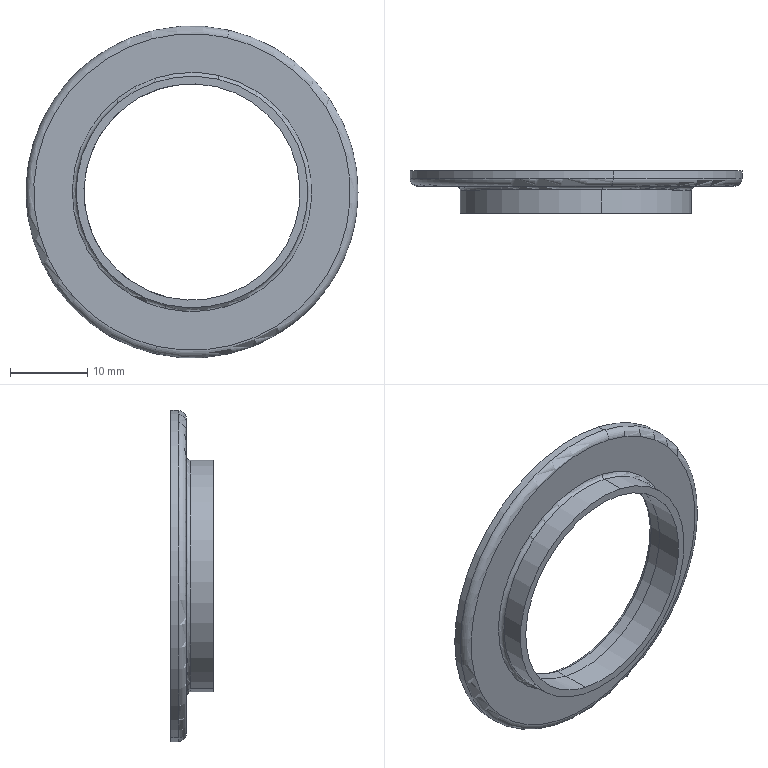Part | SolidWorks | features BaseBody 1 | 1 solid | 17 faces | box 43 x 5.5 x 43 mm | volume 1963 mm3 | cylinder 8 | torus 6 | plane 3 | commonest cylinder face diameters 28 x4 30 x2 43 x2
STEP:
#1=CARTESIAN_POINT('',(1957.589,243.9,872.98));
#2=VERTEX_POINT('',#1);
#3=CARTESIAN_POINT('',(1948.411,243.9,833.02));
#4=VERTEX_POINT('',#3);
#5=CARTESIAN_POINT('',(1953.,243.9,853.));
#6=DIRECTION('',(0.,1.,0.));
#7=DIRECTION('',(-0.9746,0.,0.2239));
#8=AXIS2_PLACEMENT_3D('',#5,#6,#7);
#9=CIRCLE('',#8,20.5);
#10=EDGE_CURVE('',#2,#4,#9,.T.);
#11=ORIENTED_EDGE('',*,*,#10,.F.);
#12=CARTESIAN_POINT('',(1957.589,243.9,872.98));
#13=CARTESIAN_POINT('',(1955.644,243.9,873.427));
#14=CARTESIAN_POINT('',(1953.644,243.9,873.637));
#15=CARTESIAN_POINT('',(1951.628,243.9,873.601));
#16=CARTESIAN_POINT('',(1947.645,243.9,873.04));
#17=CARTESIAN_POINT('',(1943.913,243.9,871.54));
#18=CARTESIAN_POINT('',(1942.148,243.9,870.565));
#19=CARTESIAN_POINT('',(1938.891,243.9,868.205));
#20=CARTESIAN_POINT('',(1936.295,243.9,865.133));
#21=CARTESIAN_POINT('',(1935.191,243.9,863.446));
#22=CARTESIAN_POINT('',(1933.416,243.9,859.837));
#23=CARTESIAN_POINT('',(1932.559,243.9,855.907));
#24=CARTESIAN_POINT('',(1932.373,243.9,853.899));
#25=CARTESIAN_POINT('',(1932.493,243.9,849.879));
#26=CARTESIAN_POINT('',(1933.574,243.9,846.005));
#27=CARTESIAN_POINT('',(1934.349,243.9,844.144));
#28=CARTESIAN_POINT('',(1936.337,243.9,840.647));
#29=CARTESIAN_POINT('',(1939.105,243.9,837.729));
#30=CARTESIAN_POINT('',(1940.661,243.9,836.446));
#31=CARTESIAN_POINT('',(1943.124,243.9,834.878));
#32=CARTESIAN_POINT('',(1945.808,243.9,833.771));
#33=CARTESIAN_POINT('',(1946.662,243.9,833.473));
#34=CARTESIAN_POINT('',(1947.531,243.9,833.222));
#35=CARTESIAN_POINT('',(1948.411,243.9,833.02));
#36=B_SPLINE_CURVE_WITH_KNOTS('',5,(#12,#13,#14,#15,#16,#17,#18,#19,#20,#21,#22,#23,#24,#25,#26,#27,#28,#29,#30,#31,#32,#33,#34,#35),.UNSPECIFIED.,.F.,.F.,(6,3,3,3,3,3,3,6),(0.,0.155,0.31,0.465,0.6199,0.7749,0.9299,1.),.UNSPECIFIED.);
#37=EDGE_CURVE('',#2,#4,#36,.T.);
#38=ORIENTED_EDGE('',*,*,#37,.T.);
#39=EDGE_LOOP('',(#11,#38));
#40=FACE_OUTER_BOUND('',#39,.T.);
#41=CARTESIAN_POINT('',(1956.47,243.9,868.107));
#42=VERTEX_POINT('',#41);
#43=CARTESIAN_POINT('',(1949.53,243.9,837.893));
#44=VERTEX_POINT('',#43);
#45=CARTESIAN_POINT('',(1956.47,243.9,868.107));
#46=CARTESIAN_POINT('',(1954.966,243.9,868.452));
#47=CARTESIAN_POINT('',(1953.419,243.9,868.61));
#48=CARTESIAN_POINT('',(1951.861,243.9,868.574));
#49=CARTESIAN_POINT('',(1948.785,243.9,868.115));
#50=CARTESIAN_POINT('',(1945.916,243.9,866.916));
#51=CARTESIAN_POINT('',(1944.563,243.9,866.141));
#52=CARTESIAN_POINT('',(1942.08,243.9,864.269));
#53=CARTESIAN_POINT('',(1940.131,243.9,861.846));
#54=CARTESIAN_POINT('',(1939.313,243.9,860.518));
#55=CARTESIAN_POINT('',(1938.025,243.9,857.688));
#56=CARTESIAN_POINT('',(1937.469,243.9,854.628));
#57=CARTESIAN_POINT('',(1937.384,243.9,853.071));
#58=CARTESIAN_POINT('',(1937.603,243.9,849.969));
#59=CARTESIAN_POINT('',(1938.576,243.9,847.015));
#60=CARTESIAN_POINT('',(1939.245,243.9,845.607));
#61=CARTESIAN_POINT('',(1940.919,243.9,842.986));
#62=CARTESIAN_POINT('',(1943.184,243.9,840.855));
#63=CARTESIAN_POINT('',(1944.444,243.9,839.937));
#64=CARTESIAN_POINT('',(1946.229,243.9,838.951));
#65=CARTESIAN_POINT('',(1948.137,243.9,838.271));
#66=CARTESIAN_POINT('',(1948.597,243.9,838.127));
#67=CARTESIAN_POINT('',(1949.061,243.9,838.001));
#68=CARTESIAN_POINT('',(1949.53,243.9,837.893));
#69=B_SPLINE_CURVE_WITH_KNOTS('',5,(#45,#46,#47,#48,#49,#50,#51,#52,#53,#54,#55,#56,#57,#58,#59,#60,#61,#62,#63,#64,#65,#66,#67,#68),.UNSPECIFIED.,.F.,.F.,(6,3,3,3,3,3,3,6),(0.,0.1584,0.3169,0.4753,0.6338,0.7922,0.9506,1.),.UNSPECIFIED.);
#70=EDGE_CURVE('',#42,#44,#69,.T.);
#71=ORIENTED_EDGE('',*,*,#70,.F.);
#72=CARTESIAN_POINT('',(1953.,243.9,853.));
#73=DIRECTION('',(0.,1.,0.));
#74=DIRECTION('',(-0.9746,0.,0.2239));
#75=AXIS2_PLACEMENT_3D('',#72,#73,#74);
#76=CIRCLE('',#75,15.5);
#77=EDGE_CURVE('',#42,#44,#76,.T.);
#78=ORIENTED_EDGE('',*,*,#77,.T.);
#79=EDGE_LOOP('',(#71,#78));
#80=FACE_BOUND('',#79,.T.);
#81=CARTESIAN_POINT('',(1953.,243.9,853.));
#82=DIRECTION('',(0.,1.,0.));
#83=DIRECTION('',(0.2239,0.,0.9746));
#84=AXIS2_PLACEMENT_3D('',#81,#82,#83);
#85=PLANE('',#84);
#86=ADVANCED_FACE('',(#40,#80),#85,.F.);
#87=ORIENTED_EDGE('',*,*,#10,.T.);
#88=CARTESIAN_POINT('',(1948.187,244.9,832.046));
#89=VERTEX_POINT('',#88);
#90=CARTESIAN_POINT('',(1948.411,244.9,833.02));
#91=DIRECTION('',(-0.9746,0.,0.2239));
#92=DIRECTION('',(0.,1.,0.));
#93=AXIS2_PLACEMENT_3D('',#90,#91,#92);
#94=CIRCLE('',#93,1.);
#95=EDGE_CURVE('',#89,#4,#94,.T.);
#96=ORIENTED_EDGE('',*,*,#95,.F.);
#97=CARTESIAN_POINT('',(1957.813,244.9,873.954));
#98=VERTEX_POINT('',#97);
#99=CARTESIAN_POINT('',(1953.,244.9,853.));
#100=DIRECTION('',(0.,1.,0.));
#101=DIRECTION('',(-0.9746,0.,0.2239));
#102=AXIS2_PLACEMENT_3D('',#99,#100,#101);
#103=CIRCLE('',#102,21.5);
#104=EDGE_CURVE('',#98,#89,#103,.T.);
#105=ORIENTED_EDGE('',*,*,#104,.F.);
#106=CARTESIAN_POINT('',(1957.589,244.9,872.98));
#107=DIRECTION('',(-0.9746,0.,0.2239));
#108=DIRECTION('',(0.,1.,0.));
#109=AXIS2_PLACEMENT_3D('',#106,#107,#108);
#110=CIRCLE('',#109,1.);
#111=EDGE_CURVE('',#2,#98,#110,.T.);
#112=ORIENTED_EDGE('',*,*,#111,.F.);
#113=EDGE_LOOP('',(#87,#96,#105,#112));
#114=FACE_OUTER_BOUND('',#113,.T.);
#115=CARTESIAN_POINT('',(1953.,244.9,853.));
#116=DIRECTION('',(0.,1.,0.));
#117=DIRECTION('',(-0.2239,0.,-0.9746));
#118=AXIS2_PLACEMENT_3D('',#115,#116,#117);
#119=TOROIDAL_SURFACE('',#118,20.5,1.);
#120=ADVANCED_FACE('',(#114),#119,.T.);
#121=CARTESIAN_POINT('',(1953.,244.9,853.));
#122=DIRECTION('',(0.,-1.,0.));
#123=DIRECTION('',(-0.9746,0.,0.2239));
#124=AXIS2_PLACEMENT_3D('',#121,#122,#123);
#125=CIRCLE('',#124,21.5);
#126=EDGE_CURVE('',#98,#89,#125,.T.);
#127=ORIENTED_EDGE('',*,*,#126,.T.);
#128=ORIENTED_EDGE('',*,*,#95,.T.);
#129=ORIENTED_EDGE('',*,*,#37,.F.);
#130=ORIENTED_EDGE('',*,*,#111,.T.);
#131=EDGE_LOOP('',(#127,#128,#129,#130));
#132=FACE_OUTER_BOUND('',#131,.T.);
#133=CARTESIAN_POINT('',(1953.,244.9,853.));
#134=DIRECTION('',(0.,1.,0.));
#135=DIRECTION('',(0.2239,0.,0.9746));
#136=AXIS2_PLACEMENT_3D('',#133,#134,#135);
#137=TOROIDAL_SURFACE('',#136,20.5,1.);
#138=ADVANCED_FACE('',(#132),#137,.T.);
#139=ORIENTED_EDGE('',*,*,#70,.T.);
#140=CARTESIAN_POINT('',(1949.642,243.4,838.381));
#141=VERTEX_POINT('',#140);
#142=CARTESIAN_POINT('',(1949.53,243.4,837.893));
#143=DIRECTION('',(0.9746,0.,-0.2239));
#144=DIRECTION('',(0.,1.,0.));
#145=AXIS2_PLACEMENT_3D('',#142,#143,#144);
#146=CIRCLE('',#145,0.5);
#147=EDGE_CURVE('',#44,#141,#146,.T.);
#148=ORIENTED_EDGE('',*,*,#147,.T.);
#149=CARTESIAN_POINT('',(1956.358,243.4,867.619));
#150=VERTEX_POINT('',#149);
#151=CARTESIAN_POINT('',(1953.,243.4,853.));
#152=DIRECTION('',(0.,-1.,0.));
#153=DIRECTION('',(-0.9746,0.,0.2239));
#154=AXIS2_PLACEMENT_3D('',#151,#152,#153);
#155=CIRCLE('',#154,15.);
#156=EDGE_CURVE('',#150,#141,#155,.T.);
#157=ORIENTED_EDGE('',*,*,#156,.F.);
#158=CARTESIAN_POINT('',(1956.47,243.4,868.107));
#159=DIRECTION('',(0.9746,0.,-0.2239));
#160=DIRECTION('',(0.,1.,0.));
#161=AXIS2_PLACEMENT_3D('',#158,#159,#160);
#162=CIRCLE('',#161,0.5);
#163=EDGE_CURVE('',#150,#42,#162,.T.);
#164=ORIENTED_EDGE('',*,*,#163,.T.);
#165=EDGE_LOOP('',(#139,#148,#157,#164));
#166=FACE_OUTER_BOUND('',#165,.T.);
#167=CARTESIAN_POINT('',(1953.,243.4,853.));
#168=DIRECTION('',(0.,1.,0.));
#169=DIRECTION('',(0.2239,0.,0.9746));
#170=AXIS2_PLACEMENT_3D('',#167,#168,#169);
#171=TOROIDAL_SURFACE('',#170,15.5,0.5);
#172=ADVANCED_FACE('',(#166),#171,.F.);
#173=CARTESIAN_POINT('',(1953.,243.4,853.));
#174=DIRECTION('',(0.,1.,0.));
#175=DIRECTION('',(-0.9746,0.,0.2239));
#176=AXIS2_PLACEMENT_3D('',#173,#174,#175);
#177=CIRCLE('',#176,15.);
#178=EDGE_CURVE('',#150,#141,#177,.T.);
#179=ORIENTED_EDGE('',*,*,#178,.T.);
#180=ORIENTED_EDGE('',*,*,#147,.F.);
#181=ORIENTED_EDGE('',*,*,#77,.F.);
#182=ORIENTED_EDGE('',*,*,#163,.F.);
#183=EDGE_LOOP('',(#179,#180,#181,#182));
#184=FACE_OUTER_BOUND('',#183,.T.);
#185=CARTESIAN_POINT('',(1953.,243.4,853.));
#186=DIRECTION('',(0.,1.,0.));
#187=DIRECTION('',(-0.2239,0.,-0.9746));
#188=AXIS2_PLACEMENT_3D('',#185,#186,#187);
#189=TOROIDAL_SURFACE('',#188,15.5,0.5);
#190=ADVANCED_FACE('',(#184),#189,.F.);
#191=ORIENTED_EDGE('',*,*,#104,.T.);
#192=CARTESIAN_POINT('',(1948.187,245.9,832.046));
#193=VERTEX_POINT('',#192);
#194=CARTESIAN_POINT('',(1948.187,240.125,832.046));
#195=DIRECTION('',(0.,-1.,0.));
#196=VECTOR('',#195,1000.);
#197=LINE('',#194,#196);
#198=EDGE_CURVE('',#193,#89,#197,.T.);
#199=ORIENTED_EDGE('',*,*,#198,.F.);
#200=CARTESIAN_POINT('',(1957.813,245.9,873.954));
#201=VERTEX_POINT('',#200);
#202=CARTESIAN_POINT('',(1953.,245.9,853.));
#203=DIRECTION('',(0.,1.,0.));
#204=DIRECTION('',(-0.9746,0.,0.2239));
#205=AXIS2_PLACEMENT_3D('',#202,#203,#204);
#206=CIRCLE('',#205,21.5);
#207=EDGE_CURVE('',#201,#193,#206,.T.);
#208=ORIENTED_EDGE('',*,*,#207,.F.);
#209=CARTESIAN_POINT('',(1957.813,240.125,873.954));
#210=DIRECTION('',(0.,1.,0.));
#211=VECTOR('',#210,1000.);
#212=LINE('',#209,#211);
#213=EDGE_CURVE('',#98,#201,#212,.T.);
#214=ORIENTED_EDGE('',*,*,#213,.F.);
#215=EDGE_LOOP('',(#191,#199,#208,#214));
#216=FACE_OUTER_BOUND('',#215,.T.);
#217=CARTESIAN_POINT('',(1953.,240.125,853.));
#218=DIRECTION('',(0.,1.,0.));
#219=DIRECTION('',(-0.2239,0.,-0.9746));
#220=AXIS2_PLACEMENT_3D('',#217,#218,#219);
#221=CYLINDRICAL_SURFACE('',#220,21.5);
#222=ADVANCED_FACE('',(#216),#221,.T.);
#223=CARTESIAN_POINT('',(1953.,245.9,853.));
#224=DIRECTION('',(0.,-1.,0.));
#225=DIRECTION('',(-0.9746,0.,0.2239));
#226=AXIS2_PLACEMENT_3D('',#223,#224,#225);
#227=CIRCLE('',#226,21.5);
#228=EDGE_CURVE('',#201,#193,#227,.T.);
#229=ORIENTED_EDGE('',*,*,#228,.T.);
#230=ORIENTED_EDGE('',*,*,#198,.T.);
#231=ORIENTED_EDGE('',*,*,#126,.F.);
#232=ORIENTED_EDGE('',*,*,#213,.T.);
#233=EDGE_LOOP('',(#229,#230,#231,#232));
#234=FACE_OUTER_BOUND('',#233,.T.);
#235=CARTESIAN_POINT('',(1953.,240.125,853.));
#236=DIRECTION('',(0.,1.,0.));
#237=DIRECTION('',(0.2239,0.,0.9746));
#238=AXIS2_PLACEMENT_3D('',#235,#236,#237);
#239=CYLINDRICAL_SURFACE('',#238,21.5);
#240=ADVANCED_FACE('',(#234),#239,.T.);
#241=ORIENTED_EDGE('',*,*,#156,.T.);
#242=CARTESIAN_POINT('',(1949.642,240.4,838.381));
#243=VERTEX_POINT('',#242);
#244=CARTESIAN_POINT('',(1949.642,240.125,838.381));
#245=DIRECTION('',(0.,-1.,0.));
#246=VECTOR('',#245,1000.);
#247=LINE('',#244,#246);
#248=EDGE_CURVE('',#141,#243,#247,.T.);
#249=ORIENTED_EDGE('',*,*,#248,.T.);
#250=CARTESIAN_POINT('',(1956.358,240.4,867.619));
#251=VERTEX_POINT('',#250);
#252=CARTESIAN_POINT('',(1953.,240.4,853.));
#253=DIRECTION('',(0.,-1.,0.));
#254=DIRECTION('',(-0.9746,0.,0.2239));
#255=AXIS2_PLACEMENT_3D('',#252,#253,#254);
#256=CIRCLE('',#255,15.);
#257=EDGE_CURVE('',#251,#243,#256,.T.);
#258=ORIENTED_EDGE('',*,*,#257,.F.);
#259=CARTESIAN_POINT('',(1956.358,240.125,867.619));
#260=DIRECTION('',(0.,1.,0.));
#261=VECTOR('',#260,1000.);
#262=LINE('',#259,#261);
#263=EDGE_CURVE('',#251,#150,#262,.T.);
#264=ORIENTED_EDGE('',*,*,#263,.T.);
#265=EDGE_LOOP('',(#241,#249,#258,#264));
#266=FACE_OUTER_BOUND('',#265,.T.);
#267=CARTESIAN_POINT('',(1953.,240.125,853.));
#268=DIRECTION('',(0.,1.,0.));
#269=DIRECTION('',(0.2239,0.,0.9746));
#270=AXIS2_PLACEMENT_3D('',#267,#268,#269);
#271=CYLINDRICAL_SURFACE('',#270,15.);
#272=ADVANCED_FACE('',(#266),#271,.T.);
#273=CARTESIAN_POINT('',(1953.,240.4,853.));
#274=DIRECTION('',(0.,1.,0.));
#275=DIRECTION('',(-0.9746,0.,0.2239));
#276=AXIS2_PLACEMENT_3D('',#273,#274,#275);
#277=CIRCLE('',#276,15.);
#278=EDGE_CURVE('',#251,#243,#277,.T.);
#279=ORIENTED_EDGE('',*,*,#278,.T.);
#280=ORIENTED_EDGE('',*,*,#248,.F.);
#281=ORIENTED_EDGE('',*,*,#178,.F.);
#282=ORIENTED_EDGE('',*,*,#263,.F.);
#283=EDGE_LOOP('',(#279,#280,#281,#282));
#284=FACE_OUTER_BOUND('',#283,.T.);
#285=CARTESIAN_POINT('',(1953.,240.125,853.));
#286=DIRECTION('',(0.,1.,0.));
#287=DIRECTION('',(-0.2239,0.,-0.9746));
#288=AXIS2_PLACEMENT_3D('',#285,#286,#287);
#289=CYLINDRICAL_SURFACE('',#288,15.);
#290=ADVANCED_FACE('',(#284),#289,.T.);
#291=ORIENTED_EDGE('',*,*,#228,.F.);
#292=ORIENTED_EDGE('',*,*,#207,.T.);
#293=EDGE_LOOP('',(#291,#292));
#294=FACE_OUTER_BOUND('',#293,.T.);
#295=CARTESIAN_POINT('',(1956.246,245.9,867.132));
#296=VERTEX_POINT('',#295);
#297=CARTESIAN_POINT('',(1949.754,245.9,838.868));
#298=VERTEX_POINT('',#297);
#299=CARTESIAN_POINT('',(1953.,245.9,853.));
#300=DIRECTION('',(0.,1.,0.));
#301=DIRECTION('',(-0.9746,0.,0.2239));
#302=AXIS2_PLACEMENT_3D('',#299,#300,#301);
#303=CIRCLE('',#302,14.5);
#304=EDGE_CURVE('',#296,#298,#303,.T.);
#305=ORIENTED_EDGE('',*,*,#304,.F.);
#306=CARTESIAN_POINT('',(1956.246,245.9,867.132));
#307=CARTESIAN_POINT('',(1954.792,245.9,867.466));
#308=CARTESIAN_POINT('',(1953.294,245.9,867.613));
#309=CARTESIAN_POINT('',(1951.786,245.9,867.565));
#310=CARTESIAN_POINT('',(1948.815,245.9,867.083));
#311=CARTESIAN_POINT('',(1946.064,245.9,865.865));
#312=CARTESIAN_POINT('',(1944.774,245.9,865.081));
#313=CARTESIAN_POINT('',(1942.425,245.9,863.2));
#314=CARTESIAN_POINT('',(1940.63,245.9,860.785));
#315=CARTESIAN_POINT('',(1939.893,245.9,859.468));
#316=CARTESIAN_POINT('',(1938.775,245.9,856.674));
#317=CARTESIAN_POINT('',(1938.4,245.9,853.688));
#318=CARTESIAN_POINT('',(1938.407,245.9,852.179));
#319=CARTESIAN_POINT('',(1938.809,245.9,849.196));
#320=CARTESIAN_POINT('',(1939.953,245.9,846.413));
#321=CARTESIAN_POINT('',(1940.701,245.9,845.102));
#322=CARTESIAN_POINT('',(1942.519,245.9,842.704));
#323=CARTESIAN_POINT('',(1944.885,245.9,840.844));
#324=CARTESIAN_POINT('',(1946.181,245.9,840.072));
#325=CARTESIAN_POINT('',(1947.707,245.9,839.413));
#326=CARTESIAN_POINT('',(1949.298,245.9,838.979));
#327=CARTESIAN_POINT('',(1949.45,245.9,838.94));
#328=CARTESIAN_POINT('',(1949.602,245.9,838.903));
#329=CARTESIAN_POINT('',(1949.754,245.9,838.868));
#330=B_SPLINE_CURVE_WITH_KNOTS('',5,(#306,#307,#308,#309,#310,#311,#312,#313,#314,#315,#316,#317,#318,#319,#320,#321,#322,#323,#324,#325,#326,#327,#328,#329),.UNSPECIFIED.,.F.,.F.,(6,3,3,3,3,3,3,6),(0.,0.1638,0.3276,0.4914,0.6552,0.819,0.9828,1.),.UNSPECIFIED.);
#331=EDGE_CURVE('',#296,#298,#330,.T.);
#332=ORIENTED_EDGE('',*,*,#331,.T.);
#333=EDGE_LOOP('',(#305,#332));
#334=FACE_BOUND('',#333,.T.);
#335=CARTESIAN_POINT('',(1953.,245.9,853.));
#336=DIRECTION('',(0.,1.,0.));
#337=DIRECTION('',(0.2239,0.,0.9746));
#338=AXIS2_PLACEMENT_3D('',#335,#336,#337);
#339=PLANE('',#338);
#340=ADVANCED_FACE('',(#294,#334),#339,.T.);
#341=ORIENTED_EDGE('',*,*,#278,.F.);
#342=ORIENTED_EDGE('',*,*,#257,.T.);
#343=EDGE_LOOP('',(#341,#342));
#344=FACE_OUTER_BOUND('',#343,.T.);
#345=CARTESIAN_POINT('',(1956.134,240.4,866.645));
#346=VERTEX_POINT('',#345);
#347=CARTESIAN_POINT('',(1949.866,240.4,839.355));
#348=VERTEX_POINT('',#347);
#349=CARTESIAN_POINT('',(1956.134,240.4,866.645));
#350=CARTESIAN_POINT('',(1954.884,240.4,866.932));
#351=CARTESIAN_POINT('',(1953.6,240.4,867.076));
#352=CARTESIAN_POINT('',(1952.306,240.4,867.072));
#353=CARTESIAN_POINT('',(1949.741,240.4,866.766));
#354=CARTESIAN_POINT('',(1947.311,240.4,865.889));
#355=CARTESIAN_POINT('',(1946.152,240.4,865.313));
#356=CARTESIAN_POINT('',(1943.987,240.4,863.904));
#357=CARTESIAN_POINT('',(1942.196,240.4,862.043));
#358=CARTESIAN_POINT('',(1941.412,240.4,861.013));
#359=CARTESIAN_POINT('',(1940.093,240.4,858.792));
#360=CARTESIAN_POINT('',(1939.311,240.4,856.33));
#361=CARTESIAN_POINT('',(1939.063,240.4,855.06));
#362=CARTESIAN_POINT('',(1938.862,240.4,852.484));
#363=CARTESIAN_POINT('',(1939.25,240.4,849.931));
#364=CARTESIAN_POINT('',(1939.59,240.4,848.681));
#365=CARTESIAN_POINT('',(1940.549,240.4,846.283));
#366=CARTESIAN_POINT('',(1942.026,240.4,844.164));
#367=CARTESIAN_POINT('',(1942.884,240.4,843.194));
#368=CARTESIAN_POINT('',(1944.666,240.4,841.593));
#369=CARTESIAN_POINT('',(1946.742,240.4,840.404));
#370=CARTESIAN_POINT('',(1947.75,240.4,839.952));
#371=CARTESIAN_POINT('',(1948.796,240.4,839.601));
#372=CARTESIAN_POINT('',(1949.866,240.4,839.355));
#373=B_SPLINE_CURVE_WITH_KNOTS('',5,(#349,#350,#351,#352,#353,#354,#355,#356,#357,#358,#359,#360,#361,#362,#363,#364,#365,#366,#367,#368,#369,#370,#371,#372),.UNSPECIFIED.,.F.,.F.,(6,3,3,3,3,3,3,6),(0.,0.1459,0.2917,0.4376,0.5835,0.7293,0.8752,1.),.UNSPECIFIED.);
#374=EDGE_CURVE('',#346,#348,#373,.T.);
#375=ORIENTED_EDGE('',*,*,#374,.F.);
#376=CARTESIAN_POINT('',(1953.,240.4,853.));
#377=DIRECTION('',(0.,1.,0.));
#378=DIRECTION('',(-0.9746,0.,0.2239));
#379=AXIS2_PLACEMENT_3D('',#376,#377,#378);
#380=CIRCLE('',#379,14.);
#381=EDGE_CURVE('',#346,#348,#380,.T.);
#382=ORIENTED_EDGE('',*,*,#381,.T.);
#383=EDGE_LOOP('',(#375,#382));
#384=FACE_BOUND('',#383,.T.);
#385=CARTESIAN_POINT('',(1953.,240.4,853.));
#386=DIRECTION('',(0.,1.,0.));
#387=DIRECTION('',(0.2239,0.,0.9746));
#388=AXIS2_PLACEMENT_3D('',#385,#386,#387);
#389=PLANE('',#388);
#390=ADVANCED_FACE('',(#344,#384),#389,.F.);
#391=ORIENTED_EDGE('',*,*,#304,.T.);
#392=CARTESIAN_POINT('',(1949.866,245.4,839.355));
#393=VERTEX_POINT('',#392);
#394=CARTESIAN_POINT('',(1949.754,245.4,838.868));
#395=DIRECTION('',(-0.9746,0.,0.2239));
#396=DIRECTION('',(0.,1.,0.));
#397=AXIS2_PLACEMENT_3D('',#394,#395,#396);
#398=CIRCLE('',#397,0.5);
#399=EDGE_CURVE('',#393,#298,#398,.T.);
#400=ORIENTED_EDGE('',*,*,#399,.F.);
#401=CARTESIAN_POINT('',(1956.134,245.4,866.645));
#402=VERTEX_POINT('',#401);
#403=CARTESIAN_POINT('',(1953.,245.4,853.));
#404=DIRECTION('',(0.,1.,0.));
#405=DIRECTION('',(-0.9746,0.,0.2239));
#406=AXIS2_PLACEMENT_3D('',#403,#404,#405);
#407=CIRCLE('',#406,14.);
#408=EDGE_CURVE('',#402,#393,#407,.T.);
#409=ORIENTED_EDGE('',*,*,#408,.F.);
#410=CARTESIAN_POINT('',(1956.246,245.4,867.132));
#411=DIRECTION('',(-0.9746,0.,0.2239));
#412=DIRECTION('',(0.,1.,0.));
#413=AXIS2_PLACEMENT_3D('',#410,#411,#412);
#414=CIRCLE('',#413,0.5);
#415=EDGE_CURVE('',#296,#402,#414,.T.);
#416=ORIENTED_EDGE('',*,*,#415,.F.);
#417=EDGE_LOOP('',(#391,#400,#409,#416));
#418=FACE_OUTER_BOUND('',#417,.T.);
#419=CARTESIAN_POINT('',(1953.,245.4,853.));
#420=DIRECTION('',(0.,1.,0.));
#421=DIRECTION('',(-0.2239,0.,-0.9746));
#422=AXIS2_PLACEMENT_3D('',#419,#420,#421);
#423=TOROIDAL_SURFACE('',#422,14.5,0.5);
#424=ADVANCED_FACE('',(#418),#423,.T.);
#425=CARTESIAN_POINT('',(1953.,245.4,853.));
#426=DIRECTION('',(0.,-1.,0.));
#427=DIRECTION('',(-0.9746,0.,0.2239));
#428=AXIS2_PLACEMENT_3D('',#425,#426,#427);
#429=CIRCLE('',#428,14.);
#430=EDGE_CURVE('',#402,#393,#429,.T.);
#431=ORIENTED_EDGE('',*,*,#430,.T.);
#432=ORIENTED_EDGE('',*,*,#399,.T.);
#433=ORIENTED_EDGE('',*,*,#331,.F.);
#434=ORIENTED_EDGE('',*,*,#415,.T.);
#435=EDGE_LOOP('',(#431,#432,#433,#434));
#436=FACE_OUTER_BOUND('',#435,.T.);
#437=CARTESIAN_POINT('',(1953.,245.4,853.));
#438=DIRECTION('',(0.,1.,0.));
#439=DIRECTION('',(0.2239,0.,0.9746));
#440=AXIS2_PLACEMENT_3D('',#437,#438,#439);
#441=TOROIDAL_SURFACE('',#440,14.5,0.5);
#442=ADVANCED_FACE('',(#436),#441,.T.);
#443=ORIENTED_EDGE('',*,*,#374,.T.);
#444=CARTESIAN_POINT('',(1949.866,243.9,839.355));
#445=VERTEX_POINT('',#444);
#446=CARTESIAN_POINT('',(1949.866,240.125,839.355));
#447=DIRECTION('',(0.,1.,0.));
#448=VECTOR('',#447,1000.);
#449=LINE('',#446,#448);
#450=EDGE_CURVE('',#348,#445,#449,.T.);
#451=ORIENTED_EDGE('',*,*,#450,.T.);
#452=CARTESIAN_POINT('',(1956.134,243.9,866.645));
#453=VERTEX_POINT('',#452);
#454=CARTESIAN_POINT('',(1953.,243.9,853.));
#455=DIRECTION('',(0.,-1.,0.));
#456=DIRECTION('',(-0.9746,0.,0.2239));
#457=AXIS2_PLACEMENT_3D('',#454,#455,#456);
#458=CIRCLE('',#457,14.);
#459=EDGE_CURVE('',#453,#445,#458,.T.);
#460=ORIENTED_EDGE('',*,*,#459,.F.);
#461=CARTESIAN_POINT('',(1956.134,240.125,866.645));
#462=DIRECTION('',(0.,-1.,0.));
#463=VECTOR('',#462,1000.);
#464=LINE('',#461,#463);
#465=EDGE_CURVE('',#453,#346,#464,.T.);
#466=ORIENTED_EDGE('',*,*,#465,.T.);
#467=EDGE_LOOP('',(#443,#451,#460,#466));
#468=FACE_OUTER_BOUND('',#467,.T.);
#469=CARTESIAN_POINT('',(1953.,240.125,853.));
#470=DIRECTION('',(0.,1.,0.));
#471=DIRECTION('',(0.2239,0.,0.9746));
#472=AXIS2_PLACEMENT_3D('',#469,#470,#471);
#473=CYLINDRICAL_SURFACE('',#472,14.);
#474=ADVANCED_FACE('',(#468),#473,.F.);
#475=CARTESIAN_POINT('',(1953.,243.9,853.));
#476=DIRECTION('',(0.,1.,0.));
#477=DIRECTION('',(-0.9746,0.,0.2239));
#478=AXIS2_PLACEMENT_3D('',#475,#476,#477);
#479=CIRCLE('',#478,14.);
#480=EDGE_CURVE('',#453,#445,#479,.T.);
#481=ORIENTED_EDGE('',*,*,#480,.T.);
#482=ORIENTED_EDGE('',*,*,#450,.F.);
#483=ORIENTED_EDGE('',*,*,#381,.F.);
#484=ORIENTED_EDGE('',*,*,#465,.F.);
#485=EDGE_LOOP('',(#481,#482,#483,#484));
#486=FACE_OUTER_BOUND('',#485,.T.);
#487=CARTESIAN_POINT('',(1953.,240.125,853.));
#488=DIRECTION('',(0.,1.,0.));
#489=DIRECTION('',(-0.2239,0.,-0.9746));
#490=AXIS2_PLACEMENT_3D('',#487,#488,#489);
#491=CYLINDRICAL_SURFACE('',#490,14.);
#492=ADVANCED_FACE('',(#486),#491,.F.);
#493=ORIENTED_EDGE('',*,*,#408,.T.);
#494=CARTESIAN_POINT('',(1949.866,240.125,839.355));
#495=DIRECTION('',(0.,1.,0.));
#496=VECTOR('',#495,1000.);
#497=LINE('',#494,#496);
#498=EDGE_CURVE('',#445,#393,#497,.T.);
#499=ORIENTED_EDGE('',*,*,#498,.F.);
#500=ORIENTED_EDGE('',*,*,#480,.F.);
#501=CARTESIAN_POINT('',(1956.134,240.125,866.645));
#502=DIRECTION('',(0.,-1.,0.));
#503=VECTOR('',#502,1000.);
#504=LINE('',#501,#503);
#505=EDGE_CURVE('',#402,#453,#504,.T.);
#506=ORIENTED_EDGE('',*,*,#505,.F.);
#507=EDGE_LOOP('',(#493,#499,#500,#506));
#508=FACE_OUTER_BOUND('',#507,.T.);
#509=CARTESIAN_POINT('',(1953.,240.125,853.));
#510=DIRECTION('',(0.,1.,0.));
#511=DIRECTION('',(-0.2239,0.,-0.9746));
#512=AXIS2_PLACEMENT_3D('',#509,#510,#511);
#513=CYLINDRICAL_SURFACE('',#512,14.);
#514=ADVANCED_FACE('',(#508),#513,.F.);
#515=ORIENTED_EDGE('',*,*,#459,.T.);
#516=ORIENTED_EDGE('',*,*,#498,.T.);
#517=ORIENTED_EDGE('',*,*,#430,.F.);
#518=ORIENTED_EDGE('',*,*,#505,.T.);
#519=EDGE_LOOP('',(#515,#516,#517,#518));
#520=FACE_OUTER_BOUND('',#519,.T.);
#521=CARTESIAN_POINT('',(1953.,240.125,853.));
#522=DIRECTION('',(0.,1.,0.));
#523=DIRECTION('',(0.2239,0.,0.9746));
#524=AXIS2_PLACEMENT_3D('',#521,#522,#523);
#525=CYLINDRICAL_SURFACE('',#524,14.);
#526=ADVANCED_FACE('',(#520),#525,.F.);
#527=CLOSED_SHELL('',(#86,#120,#138,#172,#190,#222,#240,#272,#290,#340,#390,#424,#442,#474,#492,#514,#526));
#528=MANIFOLD_SOLID_BREP('',#527);
#529=CARTESIAN_POINT('',(0.,0.,0.));
#530=DIRECTION('',(0.,0.,1.));
#531=DIRECTION('',(1.,0.,0.));
#532=AXIS2_PLACEMENT_3D('',#529,#530,#531);
#533=(LENGTH_UNIT()NAMED_UNIT(*)SI_UNIT(.MILLI.,.METRE.));
#534=UNCERTAINTY_MEASURE_WITH_UNIT(LENGTH_MEASURE(0.00001),#533,'','');
#535=(NAMED_UNIT(*)PLANE_ANGLE_UNIT()SI_UNIT($,.RADIAN.));
#536=(NAMED_UNIT(*)SI_UNIT($,.STERADIAN.)SOLID_ANGLE_UNIT());
#537=(GEOMETRIC_REPRESENTATION_CONTEXT(3)GLOBAL_UNCERTAINTY_ASSIGNED_CONTEXT((#534))GLOBAL_UNIT_ASSIGNED_CONTEXT((#533,#535,#536))REPRESENTATION_CONTEXT('',''));
#538=ADVANCED_BREP_SHAPE_REPRESENTATION('',(#528,#532),#537);